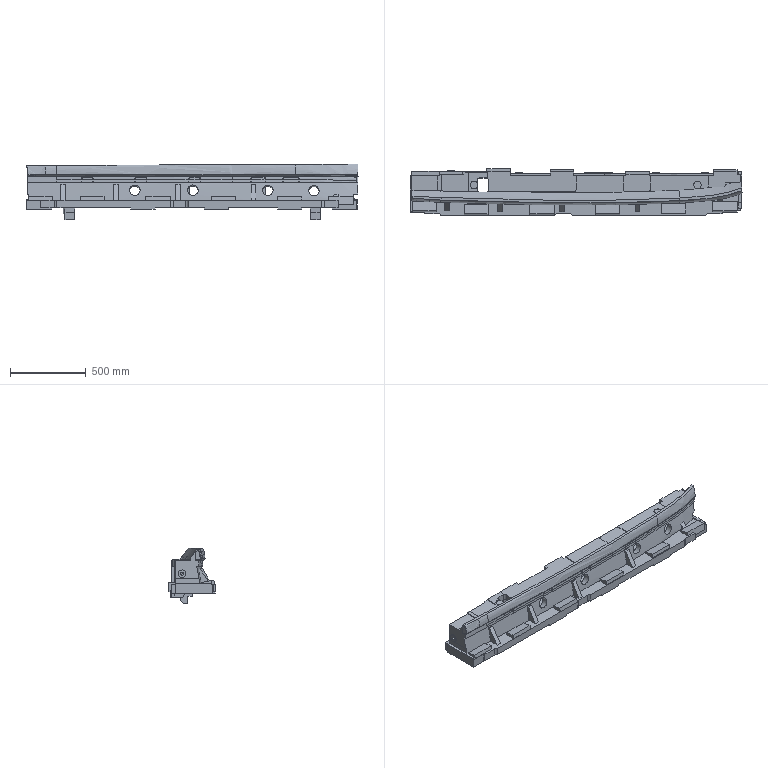Part | NX | features solid 2 | 1 solid | 452 faces | box 2197 x 305 x 370.417 mm | volume 76007140 mm3 | plane 251 | spline 156 | cylinder 42 | cone 3 | commonest cylinder face diameters 30 x17 35 x5 45 x5 20 x4 40 x4 70 x4